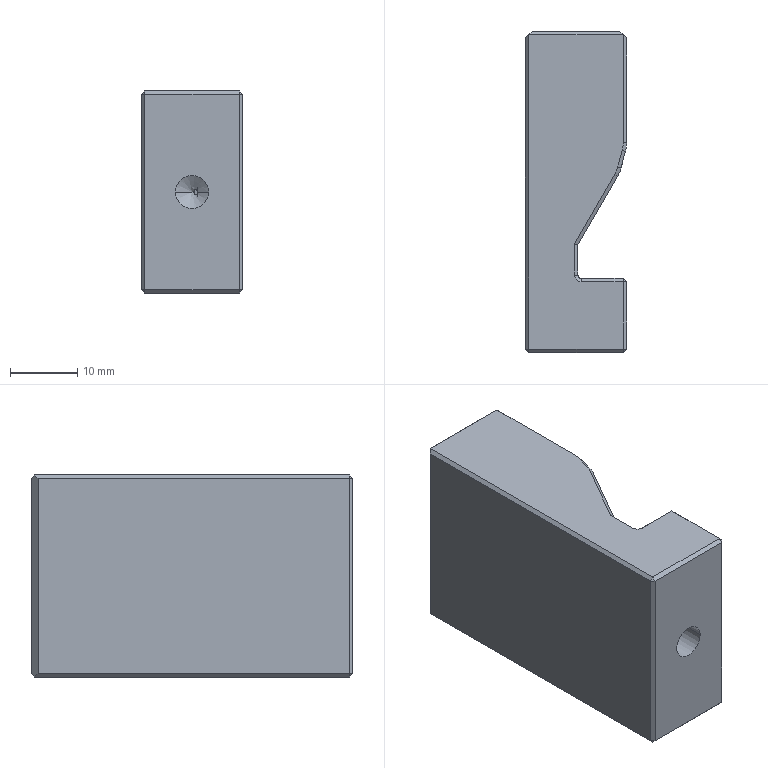Part | STEP file | chot xien con truot | 1 solid | 53 faces | box 15 x 47.7 x 30 mm | volume 18730 mm3 | plane 40 | cone 8 | cylinder 5 | commonest cylinder face diameters 4.917 x2 10 x2 1 x1